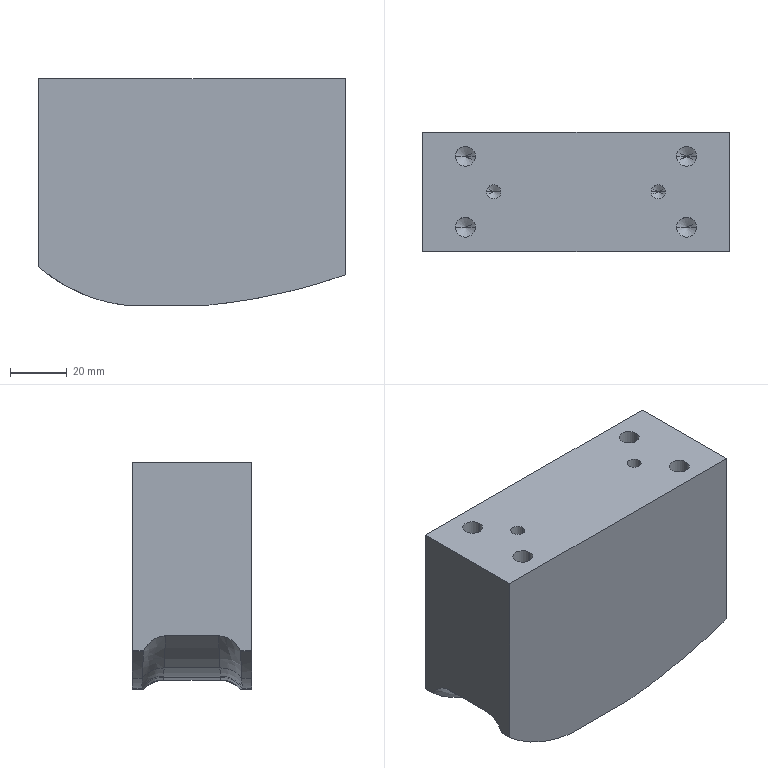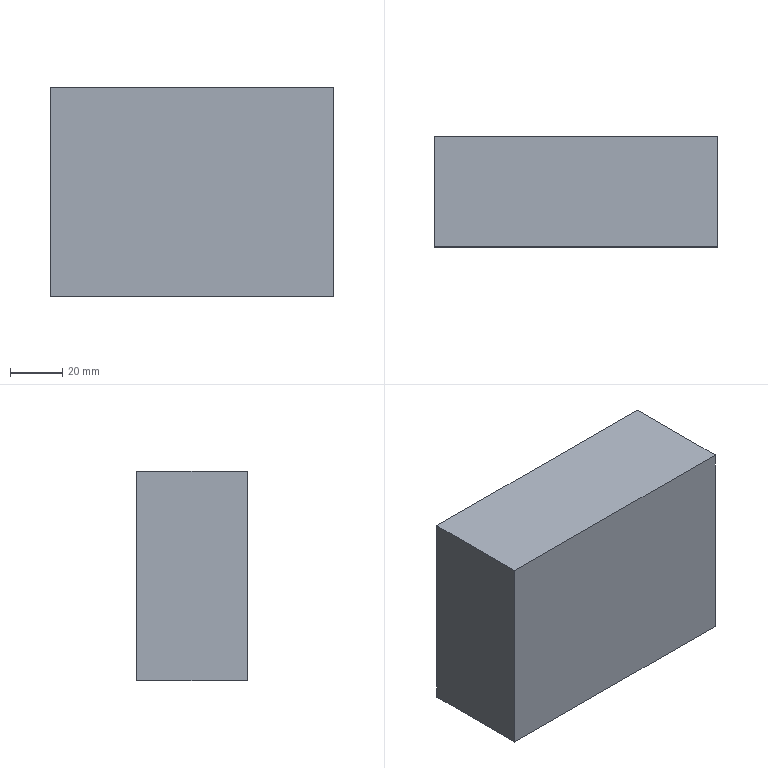CAM job | NX | 3-axis milling, drilling | part box 108 x 42 x 80.096 mm | stock box 108 x 42 x 80 mm
Tools:
number,name,description,diameter,corner_radius,flute_length,length,flutes
7,D6A45,Milling Tool-5 Parameters,6.0,0.0,3.0,3.0,2
14,4.8ZT,Drilling Tool,4.8,0.0,35.0,50.0,2
15,5.0JD,Milling Tool-5 Parameters,5.0,0.0,30.0,30.0,4
17,7.0ZT,Drilling Tool,7.0,0.0,35.0,50.0,2
5,D6R0.5,Milling Tool-5 Parameters,6.0,0.5,50.0,75.0,2
Operations:
program,operation,operation_type,tool,method,geometry_group,spindle_rpm,surface_speed,feed_per_tooth,feed_cut,feed_plunge,cut_length_mm,path_length_mm,cut_time_min,machine_time_min
1-45-85-112毛胚,DRILLING_COPY_1,Operation,D6A45,METHOD,A,5000.0,94.0,0.025,250.0,0.0,24.0,264.009,0.096,0.12
1-45-85-112毛胚,DRILLING_COPY_COPY_1,Operation,4.8ZT,METHOD,A,2000.0,15.0,0.03,120.0,0.0,38.884,198.846,0.324,0.34
1-45-85-112毛胚,DRILLING_COPY_COPY_1_COPY,Operation,5.0JD,METHOD,A,1000.0,15.0,0.0125,50.0,0.0,36.0,193.077,0.72,0.7357
1-45-85-112毛胚,DRILLING_COPY_COPY_1_COPY_1,Operation,7.0ZT,METHOD,A,2000.0,43.0,0.05,200.0,0.0,80.412,358.24,0.4021,0.4298
1-45-85-112毛胚,ZLEVEL_PROFILE_1_COPY_1_COPY,ZLevelMilling,D6A45,METHOD,A,9500.0,179.0,0.0526,1000.0,100.0,425.597,1297.791,0.4256,0.5128
2-45-85-112毛胚,FIXED_CONTOUR_COPY,SurfaceContour,D6R0.5,METHOD,B,9500.0,179.0,0.1842,3500.0,500.0,66102.244,66628.964,18.942,18.995